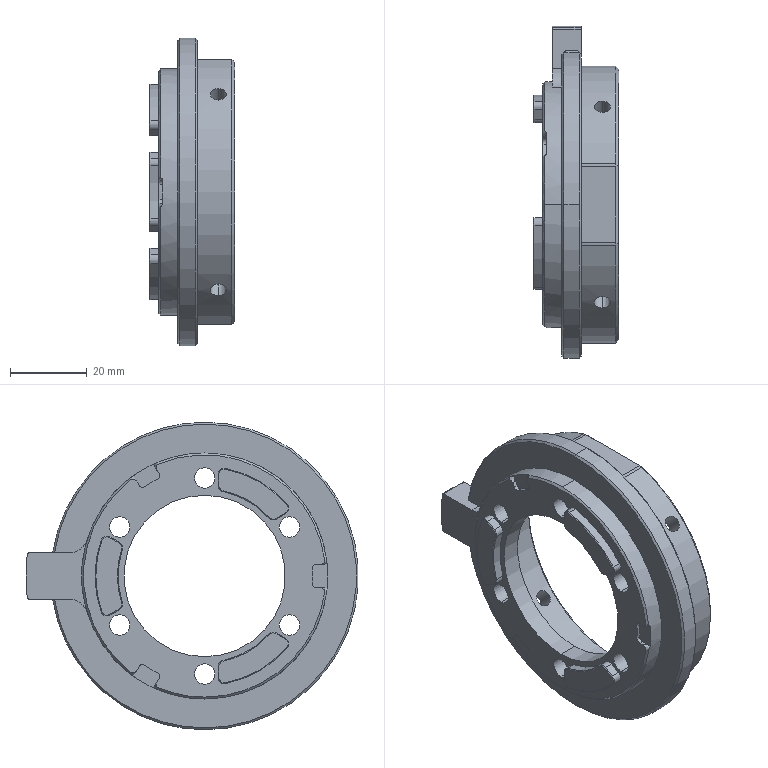NC program | NX | posted with a generic post | part box 22.3 x 86.5 x 80 mm
Lines 1 to 950 of 3025:
N10 G17 G21 G94 G90
(FLOOR_WALL_COPY , TOOL : D80)
N12 T19 M6
N14 G54
N16 G17 G0 G90 X-89. Y0. S6500 M3
N18 G43 Z30. H19
N20 Z7.
N22 G94 G1 Z4. F1500.
N24 X-86.
N26 X92.5
N28 X95.5
N30 Z7.
N32 G0 Z30.
N34 X-89.
N36 Z6.
N38 G1 Z3.
N40 X-86.
N42 X92.5
N44 X95.5
N46 Z6.
N48 G0 Z30.
N50 X-89.
N52 Z5.
N54 G1 Z2.
N56 X-86.
N58 X92.5
N60 X95.5
N62 Z5.
N64 G0 Z30.
N66 X-89.
N68 Z4.
N70 G1 Z1.
N72 X-86.
N74 X92.5
N76 X95.5
N78 Z4.
N80 G0 Z30.
N82 X-89.
N84 Z3.
N86 G1 Z0.
N88 X-86.
N90 X92.5
N92 X95.5
N94 Z3.
N96 G0 Z30.
N98 M5
(FLOOR_WALL_2 , TOOL : D10)
N100 T15 M6
N102 G54
N104 G17 G0 G90 X-45.329 Y-3.943 S9500 M3
N106 G43 Z30. H15
N108 Z0.075
N110 G94 G1 Z-0.925 F1000.
N112 X-40. Y-0.866
N114 G3 X-39.5 Y0. R1.
N116 G2 X37.908 Y11.1 R39.5 F2500.
N118 G1 X35.401
N120 G3 X35.401 Y-11.1 R-37.1
N122 G1 X37.908
N124 G2 X-39.5 Y0. R39.5
N126 G3 X-40. Y0.866 R1.
N128 G1 X-45.329 Y3.943
N130 Z0.075
N132 G0 Y-3.943 Z-0.85
N134 G1 Z-1.85 F1000.
N136 X-40. Y-0.866
N138 G3 X-39.5 Y0. R1.
N140 G2 X37.908 Y11.1 R39.5 F2500.
N142 G1 X35.401
N144 G3 X35.401 Y-11.1 R-37.1
N146 G1 X37.908
N148 G2 X-39.5 Y0. R39.5
N150 G3 X-40. Y0.866 R1.
N152 G1 X-45.329 Y3.943
N154 Z-0.85
N156 G0 Y-3.943 Z-1.775
N158 G1 Z-2.775 F1000.
N160 X-40. Y-0.866
N162 G3 X-39.5 Y0. R1.
N164 G2 X37.908 Y11.1 R39.5 F2500.
N166 G1 X35.401
N168 G3 X35.401 Y-11.1 R-37.1
N170 G1 X37.908
N172 G2 X-39.5 Y0. R39.5
N174 G3 X-40. Y0.866 R1.
N176 G1 X-45.329 Y3.943
N178 Z-1.775
N180 G0 Y-3.943 Z-2.7
N182 G1 Z-3.7 F1000.
N184 X-40. Y-0.866
N186 G3 X-39.5 Y0. R1.
N188 G2 X37.908 Y11.1 R39.5 F2500.
N190 G1 X35.401
N192 G3 X35.401 Y-11.1 R-37.1
N194 G1 X37.908
N196 G2 X-39.5 Y0. R39.5
N198 G3 X-40. Y0.866 R1.
N200 G1 X-45.329 Y3.943
N202 Z-2.7
N204 G0 Y-3.943 Z-3.625
N206 G1 Z-4.625 F1000.
N208 X-40. Y-0.866
N210 G3 X-39.5 Y0. R1.
N212 G2 X37.908 Y11.1 R39.5 F2500.
N214 G1 X35.401
N216 G3 X35.401 Y-11.1 R-37.1
N218 G1 X37.908
N220 G2 X-39.5 Y0. R39.5
N222 G3 X-40. Y0.866 R1.
N224 G1 X-45.329 Y3.943
N226 Z-3.625
N228 G0 Y-3.943 Z-4.55
N230 G1 Z-5.55 F1000.
N232 X-40. Y-0.866
N234 G3 X-39.5 Y0. R1.
N236 G2 X37.908 Y11.1 R39.5 F2500.
N238 G1 X35.401
N240 G3 X35.401 Y-11.1 R-37.1
N242 G1 X37.908
N244 G2 X-39.5 Y0. R39.5
N246 G3 X-40. Y0.866 R1.
N248 G1 X-45.329 Y3.943
N250 Z-4.55
N252 G0 Y-3.943 Z-5.475
N254 G1 Z-6.475 F1000.
N256 X-40. Y-0.866
N258 G3 X-39.5 Y0. R1.
N260 G2 X37.908 Y11.1 R39.5 F2500.
N262 G1 X35.401
N264 G3 X35.401 Y-11.1 R-37.1
N266 G1 X37.908
N268 G2 X-39.5 Y0. R39.5
N270 G3 X-40. Y0.866 R1.
N272 G1 X-45.329 Y3.943
N274 Z-5.475
N276 G0 Y-3.943 Z-6.4
N278 G1 Z-7.4 F1000.
N280 X-40. Y-0.866
N282 G3 X-39.5 Y0. R1.
N284 G2 X37.908 Y11.1 R39.5 F2500.
N286 G1 X35.401
N288 G3 X35.401 Y-11.1 R-37.1
N290 G1 X37.908
N292 G2 X-39.5 Y0. R39.5
N294 G3 X-40. Y0.866 R1.
N296 G1 X-45.329 Y3.943
N298 Z-6.4
N300 G0 Z30.
(FLOOR_WALL_2_COPY , TOOL : D10)
N302 X44.819 Y-12.
N304 Z0.02
N306 G1 Z-0.98 F1000.
N308 X44.531 Y-11.5
N310 G3 X43.665 Y-11. R1.
N312 G1 X35.432 F2500.
N314 G3 X35.432 Y11. R37.1
N316 G1 X45.659
N318 G2 X51.117 Y6.18 R5.5
N320 X51.117 Y-6.18 R50.
N322 X45.659 Y-11. R5.5
N324 G1 X43.665
N326 Y-6.
N328 X41.67
N330 G3 X41.67 Y6. R42.1
N332 G1 X45.659
N334 G2 X46.155 Y5.562 R0.5
N336 X46.155 Y-5.562 R45.
N338 X45.659 Y-6. R0.5
N340 G1 X43.665
N342 G3 X42.799 Y-6.5 R1.
N344 G1 Z0.02
N346 G0 X44.819 Y-12. Z-0.96
N348 G1 Z-1.96 F1000.
N350 X44.531 Y-11.5
N352 G3 X43.665 Y-11. R1.
N354 G1 X35.432 F2500.
N356 G3 X35.432 Y11. R37.1
N358 G1 X45.659
N360 G2 X51.117 Y6.18 R5.5
N362 X51.117 Y-6.18 R50.
N364 X45.659 Y-11. R5.5
N366 G1 X43.665
N368 Y-6.
N370 X41.67
N372 G3 X41.67 Y6. R42.1
N374 G1 X45.659
N376 G2 X46.155 Y5.562 R0.5
N378 X46.155 Y-5.562 R45.
N380 X45.659 Y-6. R0.5
N382 G1 X43.665
N384 G3 X42.799 Y-6.5 R1.
N386 G1 Z-0.96
N388 G0 X44.819 Y-12. Z-1.94
N390 G1 Z-2.94 F1000.
N392 X44.531 Y-11.5
N394 G3 X43.665 Y-11. R1.
N396 G1 X35.432 F2500.
N398 G3 X35.432 Y11. R37.1
N400 G1 X45.659
N402 G2 X51.117 Y6.18 R5.5
N404 X51.117 Y-6.18 R50.
N406 X45.659 Y-11. R5.5
N408 G1 X43.665
N410 Y-6.
N412 X41.67
N414 G3 X41.67 Y6. R42.1
N416 G1 X45.659
N418 G2 X46.155 Y5.562 R0.5
N420 X46.155 Y-5.562 R45.
N422 X45.659 Y-6. R0.5
N424 G1 X43.665
N426 G3 X42.799 Y-6.5 R1.
N428 G1 Z-1.94
N430 G0 X44.819 Y-12. Z-2.92
N432 G1 Z-3.92 F1000.
N434 X44.531 Y-11.5
N436 G3 X43.665 Y-11. R1.
N438 G1 X35.432 F2500.
N440 G3 X35.432 Y11. R37.1
N442 G1 X45.659
N444 G2 X51.117 Y6.18 R5.5
N446 X51.117 Y-6.18 R50.
N448 X45.659 Y-11. R5.5
N450 G1 X43.665
N452 Y-6.
N454 X41.67
N456 G3 X41.67 Y6. R42.1
N458 G1 X45.659
N460 G2 X46.155 Y5.562 R0.5
N462 X46.155 Y-5.562 R45.
N464 X45.659 Y-6. R0.5
N466 G1 X43.665
N468 G3 X42.799 Y-6.5 R1.
N470 G1 Z-2.92
N472 G0 X44.819 Y-12. Z-3.9
N474 G1 Z-4.9 F1000.
N476 X44.531 Y-11.5
N478 G3 X43.665 Y-11. R1.
N480 G1 X35.432 F2500.
N482 G3 X35.432 Y11. R37.1
N484 G1 X45.659
N486 G2 X51.117 Y6.18 R5.5
N488 X51.117 Y-6.18 R50.
N490 X45.659 Y-11. R5.5
N492 G1 X43.665
N494 Y-6.
N496 X41.67
N498 G3 X41.67 Y6. R42.1
N500 G1 X45.659
N502 G2 X46.155 Y5.562 R0.5
N504 X46.155 Y-5.562 R45.
N506 X45.659 Y-6. R0.5
N508 G1 X43.665
N510 G3 X42.799 Y-6.5 R1.
N512 G1 Z-3.9
N514 G0 Z30.
(FLOOR_WALL_2_COPY_COPY , TOOL : D10)
N516 X10.393 Y36.031
N518 Z0.2
N520 G1 Z-0.8 F1000.
N522 X10.511 Y35.486
N524 G3 X11.182 Y34.745 R1.
N526 G2 X13.989 Y33.713 R36.5 F2500.
N528 G1 X14.556 Y33.478
N530 X16.168 Y32.284
N532 X17.254 Y30.359
N534 X17.323 Y30.003
N536 X17.665 Y30.121
N538 X19.873 Y30.143
N540 X21.713 Y29.346
N542 X22.202 Y28.971
N544 G2 X22.202 Y-28.971 R36.5
N546 G1 X21.715 Y-29.345
N548 X19.875 Y-30.144
N550 X17.665 Y-30.122
N552 X17.322 Y-30.004
N554 X17.253 Y-30.359
N556 X16.169 Y-32.282
N558 X14.557 Y-33.477
N560 X13.989 Y-33.713
N562 G2 X-36.191 Y-4.741 R36.5
N564 G1 X-36.27 Y-4.133
N566 X-36.042 Y-2.14
N568 X-34.919 Y-0.237
N570 X-34.645 Y0.
N572 X-34.919 Y0.238
N574 X-36.041 Y2.139
N576 X-36.271 Y4.132
N578 X-36.191 Y4.741
N580 G2 X11.182 Y34.745 R36.5
N582 G1 X9.65 Y29.985
N584 G2 X12.073 Y29.095 R31.5
N586 G1 X12.336 Y28.899
N588 X12.545 Y28.53
N590 G3 X18.436 Y25.129 R5.
N592 G1 X18.859 Y25.133
N594 X19.16 Y25.003
N596 G2 X26.93 Y16.34 R31.5
N598 G3 X21.574 Y15.458 R7.7
N600 G1 X19.099 Y14.029
N602 G3 X15.616 Y5.009 R7.7
N604 G2 X15.616 Y-5.009 R16.4
N606 G3 X19.099 Y-14.029 R7.7
N608 G1 X21.574 Y-15.458
N610 G3 X26.93 Y-16.34 R7.7
N612 G1 X26.735 Y-15.36
N614 G2 X22.074 Y-14.592 R6.7
N616 G1 X19.599 Y-13.163
N618 G2 X16.569 Y-5.314 R6.7
N620 G3 X16.569 Y5.314 R17.4
N622 G2 X19.599 Y13.163 R6.7
N624 G1 X22.074 Y14.592
N626 G2 X31.756 Y10.978 R6.7
N628 X31.756 Y-10.978 R33.6
N630 X26.735 Y-15.36 R6.7
N632 G1 X26.93 Y-16.34
N634 G2 X19.16 Y-25.003 R31.5
N636 G1 X18.86 Y-25.133
N638 X18.436 Y-25.129
N640 G3 X12.544 Y-28.53 R5.
N642 G1 X12.336 Y-28.899
N644 X12.073 Y-29.095
N646 G2 X0.686 Y-31.493 R31.5
N648 G3 X2.6 Y-26.412 R7.7
N650 G1 Y-23.554
N652 G3 X0.768 Y-18.568 R7.7
N654 G1 X4.578 Y-15.331
N656 G3 X10.988 Y-11.63 R16.
N658 X16.599 Y-18.359 R12.7
N660 G1 X18.186 Y-19.275
N662 G2 X17.381 Y-20.004 R26.5
N664 G3 X8.633 Y-25.054 R10.
N666 G2 X7.6 Y-25.387 R26.5
N668 G1 Y-23.554
N670 G3 X4.578 Y-15.331 R12.7
N672 G1 X0.768 Y-18.568
N674 G3 X-3.471 Y-16.029 R7.7
N676 G2 X-12.146 Y-11.02 R16.4
N678 G3 X-21.699 Y-9.525 R7.7
N680 G1 X-24.174 Y-10.954
N682 G3 X-27.616 Y-15.152 R7.7
N684 G1 X-26.669 Y-15.473
N686 G2 X-23.674 Y-11.82 R6.7
N688 G1 X-21.199 Y-10.391
N690 G2 X-12.886 Y-11.692 R6.7
N692 G3 X-3.682 Y-17.006 R17.4
N694 G2 X1.6 Y-23.554 R6.7
N696 G1 Y-26.412
N698 G2 X-6.37 Y-32.991 R6.7
N700 X-25.386 Y-22.012 R33.6
N702 X-26.669 Y-15.473 R6.7
N704 G1 X-27.616 Y-15.152
N706 G2 X-31.233 Y-4.092 R31.5
N708 G1 X-31.196 Y-3.766
N710 X-30.98 Y-3.401
N712 G3 X-30.98 Y3.401 R5.
N714 G1 X-31.196 Y3.766
N716 X-31.233 Y4.092
N718 G2 X-27.616 Y15.152 R31.5
N720 G3 X-24.174 Y10.954 R7.7
N722 G1 X-21.699 Y9.525
N724 G3 X-16.465 Y8.619 R7.7
N726 G1 X-15.566 Y3.701
N728 G3 X-15.566 Y-3.701 R16.
N730 X-24.199 Y-5.195 R12.7
N732 G1 X-25.786 Y-6.112
N734 G2 X-26.014 Y-5.05 R26.5
N736 G3 X-26.014 Y5.051 R10.
N738 G2 X-25.786 Y6.112 R26.5
N740 G1 X-24.199 Y5.195
N742 G3 X-15.566 Y3.701 R12.7
N744 G1 X-16.465 Y8.619
N746 G3 X-12.146 Y11.02 R7.7
N748 G2 X-3.471 Y16.029 R16.4
N750 G3 X2.6 Y23.554 R7.7
N752 G1 Y26.412
N754 G3 X0.686 Y31.493 R7.7
N756 G1 X-0.065 Y30.833
N758 G2 X1.6 Y26.412 R6.7
N760 G1 Y23.554
N762 G2 X-3.682 Y17.006 R6.7
N764 G3 X-12.886 Y11.692 R17.4
N766 G2 X-21.199 Y10.391 R6.7
N768 G1 X-23.674 Y11.82
N770 G2 X-25.386 Y22.012 R6.7
N772 X-6.37 Y32.991 R33.6
N774 X-0.065 Y30.833 R6.7
N776 G1 X0.686 Y31.493
N778 G2 X9.65 Y29.985 R31.5
N780 G1 X8.118 Y25.226
N782 G2 X8.633 Y25.054 R26.5
N784 G3 X17.381 Y20.004 R10.
N786 G2 X18.186 Y19.275 R26.5
N788 G1 X16.599 Y18.359
N790 G3 X10.988 Y11.63 R12.7
N792 X4.578 Y15.331 R16.
N794 X7.6 Y23.554 R12.7
N796 G1 Y25.387
N798 G2 X8.118 Y25.226 R26.5
N800 G3 X9.096 Y25.436 R1.
N802 G1 Z0.2
N804 G0 X10.393 Y36.031 Z-0.6
N806 G1 Z-1.6 F1000.
N808 X10.511 Y35.486
N810 G3 X11.182 Y34.745 R1.
N812 G2 X13.989 Y33.713 R36.5 F2500.
N814 G1 X14.556 Y33.478
N816 X16.168 Y32.284
N818 X17.254 Y30.359
N820 X17.323 Y30.003
N822 X17.665 Y30.121
N824 X19.873 Y30.143
N826 X21.713 Y29.346
N828 X22.202 Y28.971
N830 G2 X22.202 Y-28.971 R36.5
N832 G1 X21.715 Y-29.345
N834 X19.875 Y-30.144
N836 X17.665 Y-30.122
N838 X17.322 Y-30.004
N840 X17.253 Y-30.359
N842 X16.169 Y-32.282
N844 X14.557 Y-33.477
N846 X13.989 Y-33.713
N848 G2 X-36.191 Y-4.741 R36.5
N850 G1 X-36.27 Y-4.133
N852 X-36.042 Y-2.14
N854 X-34.919 Y-0.237
N856 X-34.645 Y0.
N858 X-34.919 Y0.238
N860 X-36.041 Y2.139
N862 X-36.271 Y4.132
N864 X-36.191 Y4.741
N866 G2 X11.182 Y34.745 R36.5
N868 G1 X9.65 Y29.985
N870 G2 X12.073 Y29.095 R31.5
N872 G1 X12.336 Y28.899
N874 X12.545 Y28.53
N876 G3 X18.436 Y25.129 R5.
N878 G1 X18.859 Y25.133
N880 X19.16 Y25.003
N882 G2 X26.93 Y16.34 R31.5
N884 G3 X21.574 Y15.458 R7.7
N886 G1 X19.099 Y14.029
N888 G3 X15.616 Y5.009 R7.7
N890 G2 X15.616 Y-5.009 R16.4
N892 G3 X19.099 Y-14.029 R7.7
N894 G1 X21.574 Y-15.458
N896 G3 X26.93 Y-16.34 R7.7
N898 G1 X26.735 Y-15.36
N900 G2 X22.074 Y-14.592 R6.7
N902 G1 X19.599 Y-13.163
N904 G2 X16.569 Y-5.314 R6.7
N906 G3 X16.569 Y5.314 R17.4
N908 G2 X19.599 Y13.163 R6.7
N910 G1 X22.074 Y14.592
N912 G2 X31.756 Y10.978 R6.7
N914 X31.756 Y-10.978 R33.6
N916 X26.735 Y-15.36 R6.7
N918 G1 X26.93 Y-16.34
N920 G2 X19.16 Y-25.003 R31.5
N922 G1 X18.86 Y-25.133
N924 X18.436 Y-25.129
N926 G3 X12.544 Y-28.53 R5.
N928 G1 X12.336 Y-28.899
N930 X12.073 Y-29.095
N932 G2 X0.686 Y-31.493 R31.5
N934 G3 X2.6 Y-26.412 R7.7
N936 G1 Y-23.554
N938 G3 X0.768 Y-18.568 R7.7
N940 G1 X4.578 Y-15.331
N942 G3 X10.988 Y-11.63 R16.
N944 X16.599 Y-18.359 R12.7
N946 G1 X18.186 Y-19.275
N948 G2 X17.381 Y-20.004 R26.5
N950 G3 X8.633 Y-25.054 R10.
N952 G2 X7.6 Y-25.387 R26.5
N954 G1 Y-23.554
N956 G3 X4.578 Y-15.331 R12.7
N958 G1 X0.768 Y-18.568
N960 G3 X-3.471 Y-16.029 R7.7
N962 G2 X-12.146 Y-11.02 R16.4
N964 G3 X-21.699 Y-9.525 R7.7
N966 G1 X-24.174 Y-10.954
N968 G3 X-27.616 Y-15.152 R7.7
N970 G1 X-26.669 Y-15.473
N972 G2 X-23.674 Y-11.82 R6.7
N974 G1 X-21.199 Y-10.391
N976 G2 X-12.886 Y-11.692 R6.7
N978 G3 X-3.682 Y-17.006 R17.4
N980 G2 X1.6 Y-23.554 R6.7
N982 G1 Y-26.412
N984 G2 X-6.37 Y-32.991 R6.7
N986 X-25.386 Y-22.012 R33.6
N988 X-26.669 Y-15.473 R6.7
N990 G1 X-27.616 Y-15.152
N992 G2 X-31.233 Y-4.092 R31.5
N994 G1 X-31.196 Y-3.766
N996 X-30.98 Y-3.401
N998 G3 X-30.98 Y3.401 R5.
N1000 G1 X-31.196 Y3.766
N1002 X-31.233 Y4.092
N1004 G2 X-27.616 Y15.152 R31.5
N1006 G3 X-24.174 Y10.954 R7.7
N1008 G1 X-21.699 Y9.525
N1010 G3 X-16.465 Y8.619 R7.7
N1012 G1 X-15.566 Y3.701
N1014 G3 X-15.566 Y-3.701 R16.
N1016 X-24.199 Y-5.195 R12.7
N1018 G1 X-25.786 Y-6.112
N1020 G2 X-26.014 Y-5.05 R26.5
N1022 G3 X-26.014 Y5.051 R10.
N1024 G2 X-25.786 Y6.112 R26.5
N1026 G1 X-24.199 Y5.195
N1028 G3 X-15.566 Y3.701 R12.7
N1030 G1 X-16.465 Y8.619
N1032 G3 X-12.146 Y11.02 R7.7
N1034 G2 X-3.471 Y16.029 R16.4
N1036 G3 X2.6 Y23.554 R7.7
N1038 G1 Y26.412
N1040 G3 X0.686 Y31.493 R7.7
N1042 G1 X-0.065 Y30.833
N1044 G2 X1.6 Y26.412 R6.7
N1046 G1 Y23.554
N1048 G2 X-3.682 Y17.006 R6.7
N1050 G3 X-12.886 Y11.692 R17.4
N1052 G2 X-21.199 Y10.391 R6.7
N1054 G1 X-23.674 Y11.82
N1056 G2 X-25.386 Y22.012 R6.7
N1058 X-6.37 Y32.991 R33.6
N1060 X-0.065 Y30.833 R6.7
N1062 G1 X0.686 Y31.493
N1064 G2 X9.65 Y29.985 R31.5
N1066 G1 X8.118 Y25.226
N1068 G2 X8.633 Y25.054 R26.5
N1070 G3 X17.381 Y20.004 R10.
N1072 G2 X18.186 Y19.275 R26.5
N1074 G1 X16.599 Y18.359
N1076 G3 X10.988 Y11.63 R12.7
N1078 X4.578 Y15.331 R16.
N1080 X7.6 Y23.554 R12.7
N1082 G1 Y25.387
N1084 G2 X8.118 Y25.226 R26.5
N1086 G3 X9.096 Y25.436 R1.
N1088 G1 Z-0.6
N1090 G0 X10.393 Y36.031 Z-1.4
N1092 G1 Z-2.4 F1000.
N1094 X10.511 Y35.486
N1096 G3 X11.182 Y34.745 R1.
N1098 G2 X13.989 Y33.713 R36.5 F2500.
N1100 G1 X14.556 Y33.478
N1102 X16.168 Y32.284
N1104 X17.254 Y30.359
N1106 X17.323 Y30.003
N1108 X17.665 Y30.121
N1110 X19.873 Y30.143
N1112 X21.713 Y29.346
N1114 X22.202 Y28.971
N1116 G2 X22.202 Y-28.971 R36.5
N1118 G1 X21.715 Y-29.345
N1120 X19.875 Y-30.144
N1122 X17.665 Y-30.122
N1124 X17.322 Y-30.004
N1126 X17.253 Y-30.359
N1128 X16.169 Y-32.282
N1130 X14.557 Y-33.477
N1132 X13.989 Y-33.713
N1134 G2 X-36.191 Y-4.741 R36.5
N1136 G1 X-36.27 Y-4.133
N1138 X-36.042 Y-2.14
N1140 X-34.919 Y-0.237
N1142 X-34.645 Y0.
N1144 X-34.919 Y0.238
N1146 X-36.041 Y2.139
N1148 X-36.271 Y4.132
N1150 X-36.191 Y4.741
N1152 G2 X11.182 Y34.745 R36.5
N1154 G1 X9.65 Y29.985
N1156 G2 X12.073 Y29.095 R31.5
N1158 G1 X12.336 Y28.899
N1160 X12.545 Y28.53
N1162 G3 X18.436 Y25.129 R5.
N1164 G1 X18.859 Y25.133
N1166 X19.16 Y25.003
N1168 G2 X26.93 Y16.34 R31.5
N1170 G3 X21.574 Y15.458 R7.7
N1172 G1 X19.099 Y14.029
N1174 G3 X15.616 Y5.009 R7.7
N1176 G2 X15.616 Y-5.009 R16.4
N1178 G3 X19.099 Y-14.029 R7.7
N1180 G1 X21.574 Y-15.458
N1182 G3 X26.93 Y-16.34 R7.7
N1184 G1 X26.735 Y-15.36
N1186 G2 X22.074 Y-14.592 R6.7
N1188 G1 X19.599 Y-13.163
N1190 G2 X16.569 Y-5.314 R6.7
N1192 G3 X16.569 Y5.314 R17.4
N1194 G2 X19.599 Y13.163 R6.7
N1196 G1 X22.074 Y14.592
N1198 G2 X31.756 Y10.978 R6.7
N1200 X31.756 Y-10.978 R33.6
N1202 X26.735 Y-15.36 R6.7
N1204 G1 X26.93 Y-16.34
N1206 G2 X19.16 Y-25.003 R31.5
N1208 G1 X18.86 Y-25.133
N1210 X18.436 Y-25.129
N1212 G3 X12.544 Y-28.53 R5.
N1214 G1 X12.336 Y-28.899
N1216 X12.073 Y-29.095
N1218 G2 X0.686 Y-31.493 R31.5
N1220 G3 X2.6 Y-26.412 R7.7
N1222 G1 Y-23.554
N1224 G3 X0.768 Y-18.568 R7.7
N1226 G1 X4.578 Y-15.331
N1228 G3 X10.988 Y-11.63 R16.
N1230 X16.599 Y-18.359 R12.7
N1232 G1 X18.186 Y-19.275
N1234 G2 X17.381 Y-20.004 R26.5
N1236 G3 X8.633 Y-25.054 R10.
N1238 G2 X7.6 Y-25.387 R26.5
N1240 G1 Y-23.554
N1242 G3 X4.578 Y-15.331 R12.7
N1244 G1 X0.768 Y-18.568
N1246 G3 X-3.471 Y-16.029 R7.7
N1248 G2 X-12.146 Y-11.02 R16.4
N1250 G3 X-21.699 Y-9.525 R7.7
N1252 G1 X-24.174 Y-10.954
N1254 G3 X-27.616 Y-15.152 R7.7
N1256 G1 X-26.669 Y-15.473
N1258 G2 X-23.674 Y-11.82 R6.7
N1260 G1 X-21.199 Y-10.391
N1262 G2 X-12.886 Y-11.692 R6.7
N1264 G3 X-3.682 Y-17.006 R17.4
N1266 G2 X1.6 Y-23.554 R6.7
N1268 G1 Y-26.412
N1270 G2 X-6.37 Y-32.991 R6.7
N1272 X-25.386 Y-22.012 R33.6
N1274 X-26.669 Y-15.473 R6.7
N1276 G1 X-27.616 Y-15.152
N1278 G2 X-31.233 Y-4.092 R31.5
N1280 G1 X-31.196 Y-3.766
N1282 X-30.98 Y-3.401
N1284 G3 X-30.98 Y3.401 R5.
N1286 G1 X-31.196 Y3.766
N1288 X-31.233 Y4.092
N1290 G2 X-27.616 Y15.152 R31.5
N1292 G3 X-24.174 Y10.954 R7.7
N1294 G1 X-21.699 Y9.525
N1296 G3 X-16.465 Y8.619 R7.7
N1298 G1 X-15.566 Y3.701
N1300 G3 X-15.566 Y-3.701 R16.
N1302 X-24.199 Y-5.195 R12.7
N1304 G1 X-25.786 Y-6.112
N1306 G2 X-26.014 Y-5.05 R26.5
N1308 G3 X-26.014 Y5.051 R10.
N1310 G2 X-25.786 Y6.112 R26.5
N1312 G1 X-24.199 Y5.195
N1314 G3 X-15.566 Y3.701 R12.7
N1316 G1 X-16.465 Y8.619
N1318 G3 X-12.146 Y11.02 R7.7
N1320 G2 X-3.471 Y16.029 R16.4
N1322 G3 X2.6 Y23.554 R7.7
N1324 G1 Y26.412
N1326 G3 X0.686 Y31.493 R7.7
N1328 G1 X-0.065 Y30.833
N1330 G2 X1.6 Y26.412 R6.7
N1332 G1 Y23.554
N1334 G2 X-3.682 Y17.006 R6.7
N1336 G3 X-12.886 Y11.692 R17.4
N1338 G2 X-21.199 Y10.391 R6.7
N1340 G1 X-23.674 Y11.82
N1342 G2 X-25.386 Y22.012 R6.7
N1344 X-6.37 Y32.991 R33.6
N1346 X-0.065 Y30.833 R6.7
N1348 G1 X0.686 Y31.493
N1350 G2 X9.65 Y29.985 R31.5
N1352 G1 X8.118 Y25.226
N1354 G2 X8.633 Y25.054 R26.5
N1356 G3 X17.381 Y20.004 R10.
N1358 G2 X18.186 Y19.275 R26.5
N1360 G1 X16.599 Y18.359
N1362 G3 X10.988 Y11.63 R12.7
N1364 X4.578 Y15.331 R16.
N1366 X7.6 Y23.554 R12.7
N1368 G1 Y25.387
N1370 G2 X8.118 Y25.226 R26.5
N1372 G3 X9.096 Y25.436 R1.
N1374 G1 Z-1.4
N1376 G0 Z30.
N1378 M5
(FLOOR_WALL_1_COPY_1 , TOOL : D10JING)
N1380 T14 M6
N1382 G54
N1384 G17 G0 G90 X43.867 Y-14. S9500 M3
N1386 G43 Z30. H14
N1388 Z-2.
N1390 G94 G1 Z-5. F1250.
N1392 Y-11.
N1394 X35.85
N1396 G3 X35.85 Y11. R37.5
N1398 G1 X45.659
N1400 G2 X51.117 Y6.18 R5.5
N1402 X51.117 Y-6.18 R50.
N1404 X45.659 Y-11. R5.5
N1406 G1 X43.867
N1408 Y-6.
N1410 X42.074
N1412 G3 X42.074 Y6. R42.5
N1414 G1 X45.659
N1416 G2 X46.155 Y5.562 R0.5
N1418 X46.155 Y-5.562 R45.
N1420 X45.659 Y-6. R0.5
N1422 G1 X43.867
N1424 Y-14.
N1426 Z-2.
N1428 G0 Z30.
N1430 X37.105 Y14.939
N1432 Z-2.
N1434 G1 Z-5.
N1436 X34.435 Y13.864
N1438 X35.327 Y11.
N1440 G2 X35.327 Y-11. R37.
N1442 G1 X34.435 Y-13.864
N1444 X37.105 Y-14.939
N1446 Z-2.
N1448 G0 Z30.
N1450 X-47.5 Y0.
N1452 Z-4.5
N1454 G1 Z-7.5
N1456 X-44.5
N1458 G2 X42.988 Y11.5 R44.5
N1460 G1 X35.693
N1462 G3 X35.693 Y-11.5 R-37.5
N1464 G1 X42.988
N1466 G2 X-44.5 Y0. R44.5
N1468 G1 X-47.5
N1470 Z-4.5
N1472 G0 Z30.
N1474 X46.368 Y-13.97
N1476 Z-4.5
N1478 G1 Z-7.5
N1480 X46.119 Y-11.
N1482 X43.119
N1484 X35.327
N1486 G2 X35.327 Y11. R-37.
N1488 G1 X43.119
N1490 X46.119
N1492 X46.368 Y13.97
N1494 Z-4.5
N1496 G0 Z30.
(FLOOR_WALL_1_COPY_COPY , TOOL : D10JING)
N1498 X11.914 Y12.554
N1500 Z3.5
N1502 G1 X12.071 Y12.906 Z3.397
N1504 X12.725 Y14.037 Z3.047
N1506 X13.497 Y15.091 Z2.697
N1508 X14.377 Y16.056 Z2.347
N1510 X15.356 Y16.922 Z1.996
N1512 X16.421 Y17.679 Z1.646
N1514 X18.561 Y18.914 Z0.984
N1516 X18.041 Y19.424 Z0.789
N1518 X17.932 Y19.525 Z0.749
N1520 X17.382 Y20.003 Z0.554
N1522 X16.935 Y20. Z0.434
N1524 X15.728 Y20.121 Z0.109
N1526 X14.545 Y20.386 Z-0.216
N1528 X13.402 Y20.792 Z-0.54
N1530 X12.317 Y21.334 Z-0.865
N1532 X11.306 Y22.003 Z-1.19
N1534 X10.382 Y22.789 Z-1.515
N1536 X9.561 Y23.681 Z-1.84
N1538 X8.854 Y24.666 Z-2.165
N1540 X8.632 Y25.055 Z-2.285
N1542 X8.253 Y25.185 Z-2.392
N1544 X7.87 Y25.304 Z-2.5
N1546 G3 X7.1 Y25.531 R26.5
N1548 G1 Y23.554
N1550 G2 X4.046 Y15.48 R12.2
N1552 X11.383 Y11.244 R16.
N1554 X16.849 Y17.926 R12.2
N1556 G1 X18.561 Y18.914
N1558 G3 X17.382 Y20.003 R26.5
N1560 G2 X8.632 Y25.055 R10.
N1562 G3 X7.87 Y25.304 R26.5
N1564 G1 X9.355 Y30.079
N1566 G3 X-0.006 Y31.5 R31.5
N1568 G2 X2.1 Y26.412 R7.2
N1570 G1 Y23.554
N1572 G2 X-3.576 Y16.517 R7.2
N1574 G3 X-12.516 Y11.356 R16.9
N1576 G2 X-16.421 Y9.137 R7.2
N1578 G1 X-15.429 Y4.236
N1580 G2 X-23.949 Y5.628 R12.2
N1582 G1 X-25.661 Y6.617
N1584 G3 X-26.014 Y5.052 R26.5
N1586 G2 X-26.014 Y-5.052 R10.
N1588 G3 X-25.661 Y-6.617 R26.5
N1590 G1 X-23.949 Y-5.628
N1592 G2 X-15.429 Y-4.236 R12.2
N1594 X-15.429 Y4.236 R16.
N1596 G1 X-16.421 Y9.137
N1598 G2 X-21.449 Y9.958 R7.2
N1600 G1 X-23.924 Y11.387
N1602 G2 X-27.277 Y15.755 R7.2
N1604 G3 X-31.233 Y4.092 R31.5
N1606 G1 X-31.219 Y3.845
N1608 X-31.125 Y3.616
N1610 X-30.704 Y3.078
N1612 G2 X-30.705 Y-3.079 R5.
N1614 G1 X-31.125 Y-3.616
N1616 X-31.219 Y-3.845
N1618 X-31.233 Y-4.092
N1620 G3 X-27.277 Y-15.755 R31.5
N1622 G2 X-23.924 Y-11.387 R7.2
N1624 G1 X-21.449 Y-9.958
N1626 G2 X-12.516 Y-11.356 R7.2
N1628 G3 X-3.576 Y-16.517 R16.9
N1630 G2 X0.298 Y-18.789 R7.2
N1632 G1 X4.046 Y-15.48
N1634 G2 X7.1 Y-23.554 R12.2
N1636 G1 Y-25.531
N1638 G3 X8.632 Y-25.055 R26.5
N1640 G2 X17.382 Y-20.003 R10.
N1642 G3 X18.561 Y-18.914 R26.5
N1644 G1 X16.849 Y-17.926
N1646 G2 X11.383 Y-11.244 R12.2
N1648 X4.046 Y-15.48 R16.
N1650 G1 X0.298 Y-18.789
N1652 G2 X2.1 Y-23.554 R7.2
N1654 G1 Y-26.412
N1656 G2 X-0.006 Y-31.5 R7.2
N1658 G3 X12.073 Y-29.095 R31.5
N1660 G1 X12.28 Y-28.959
N1662 X12.43 Y-28.763
N1664 X12.686 Y-28.13
N1666 G2 X18.019 Y-25.052 R5.
N1668 G1 X18.694 Y-25.147
N1670 X18.939 Y-25.114
N1672 X19.16 Y-25.003
N1674 G3 X27.283 Y-15.745 R31.5
N1676 G2 X21.824 Y-15.025 R7.2
N1678 G1 X19.349 Y-13.596
N1680 G2 X16.093 Y-5.161 R7.2
N1682 G3 X16.093 Y5.161 R16.9
N1684 G2 X19.349 Y13.596 R7.2
N1686 G1 X21.824 Y15.025
N1688 G2 X27.283 Y15.745 R7.2
N1690 G3 X19.16 Y25.003 R31.5
N1692 G1 X18.939 Y25.114
N1694 X18.694 Y25.146
N1696 X18.018 Y25.051
N1698 G2 X12.686 Y28.131 R5.
N1700 G1 X12.431 Y28.763
N1702 X12.28 Y28.959
N1704 X12.073 Y29.095
N1706 G3 X9.355 Y30.079 R31.5
N1708 G1 X10.839 Y34.853
N1710 G3 X-36.191 Y4.741 R36.5
N1712 G1 X-36.251 Y4.278
N1714 X-36.164 Y2.716
N1716 X-35.484 Y1.075
N1718 X-34.644 Y0.
N1720 X-35.485 Y-1.075
N1722 X-36.164 Y-2.719
N1724 X-36.251 Y-4.279
N1726 X-36.191 Y-4.741
N1728 G3 X13.989 Y-33.713 R36.5
N1730 G1 X14.421 Y-33.534
N1732 X15.729 Y-32.677
N1734 X16.811 Y-31.267
N1736 X17.322 Y-30.003
N1738 X18.674 Y-30.193
N1740 X20.437 Y-29.96
N1742 X21.831 Y-29.255
N1744 X22.202 Y-28.971
N1746 G3 X22.202 Y28.971 R36.5
N1748 G1 X21.83 Y29.256
N1750 X20.434 Y29.96
N1752 X18.673 Y30.193
N1754 X17.322 Y30.003
N1756 X16.811 Y31.268
N1758 X15.727 Y32.679
N1760 X14.42 Y33.534
N1762 X13.989 Y33.713
N1764 G3 X10.839 Y34.853 R36.5
N1766 G1 X11.73 Y37.718
N1768 Z0.5
N1770 G0 Z30.
N1772 X-6.304 Y38.994
N1774 Z0.5
N1776 G1 Z-2.5
N1778 X-5.738 Y33.082
N1780 G2 X1.6 Y26.412 R6.7
N1782 G1 Y23.554
N1784 G2 X-3.682 Y17.006 R6.7
N1786 G3 X-12.886 Y11.692 R17.4
N1788 G2 X-21.199 Y10.391 R6.7
N1790 G1 X-23.674 Y11.82
N1792 G2 X-25.386 Y22.012 R6.7
N1794 X-6.37 Y32.991 R33.6
N1796 X-5.738 Y33.082 R6.7
N1798 G1 X-6.071 Y36.566
N1800 Z0.5
N1802 G0 Z30.
N1804 X19.086 Y16.908
N1806 Z0.5
N1808 G1 Z-2.5
N1810 X20.836 Y13.877
N1812 X22.074 Y14.592
N1814 G2 X31.756 Y10.978 R6.7
N1816 X31.756 Y-10.978 R33.6
N1818 X22.074 Y-14.592 R6.7
N1820 G1 X19.599 Y-13.163
N1822 G2 X16.569 Y-5.314 R6.7
N1824 G3 X16.569 Y5.314 R17.4
N1826 G2 X19.599 Y13.163 R6.7
N1828 G1 X20.836 Y13.877
N1830 X19.086 Y16.908
N1832 Z0.5
N1834 G0 Z30.
N1836 X5.1 Y-24.983
N1838 Z0.5
N1840 G1 Z-2.5
N1842 X1.6
N1844 Y-26.412
N1846 G2 X-6.37 Y-32.991 R6.7
N1848 X-25.386 Y-22.012 R33.6
N1850 X-23.674 Y-11.82 R6.7
N1852 G1 X-21.199 Y-10.391
N1854 G2 X-12.886 Y-11.692 R6.7
N1856 G3 X-3.682 Y-17.006 R17.4
N1858 G2 X1.6 Y-23.554 R6.7
N1860 G1 Y-24.983
N1862 X5.1
N1864 Z0.5
N1866 G0 Z30.
N1868 M5